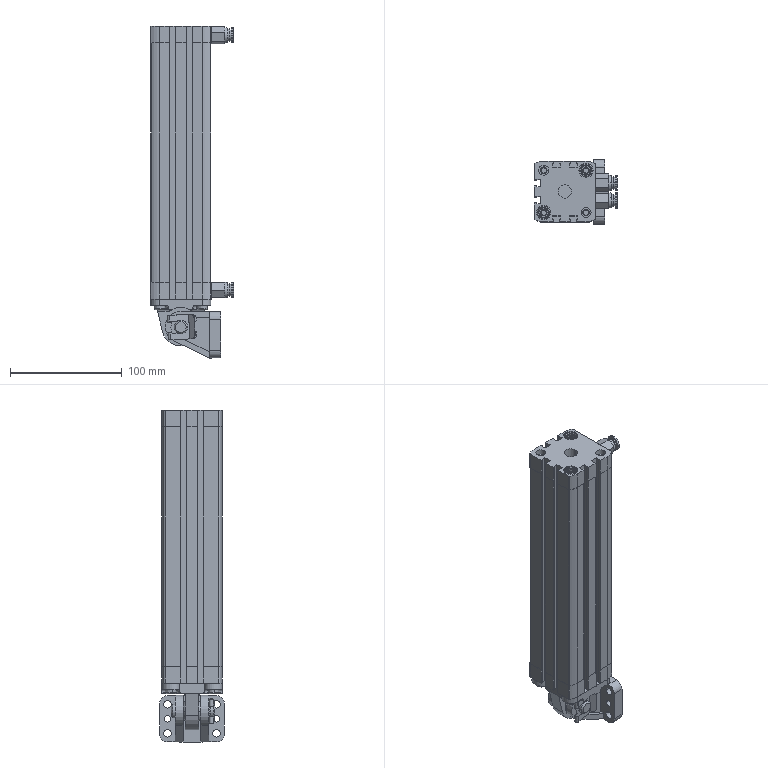Part | SolidWorks | 10 solids | 858 faces | box 74.5 x 58 x 297.75 mm | volume 433626 mm3 | plane 428 | cylinder 266 | cone 140 | torus 20 | spline 4 | commonest cylinder face diameters 2 x37 0.4 x24 4.917 x16 6 x16 12 x15 9 x13